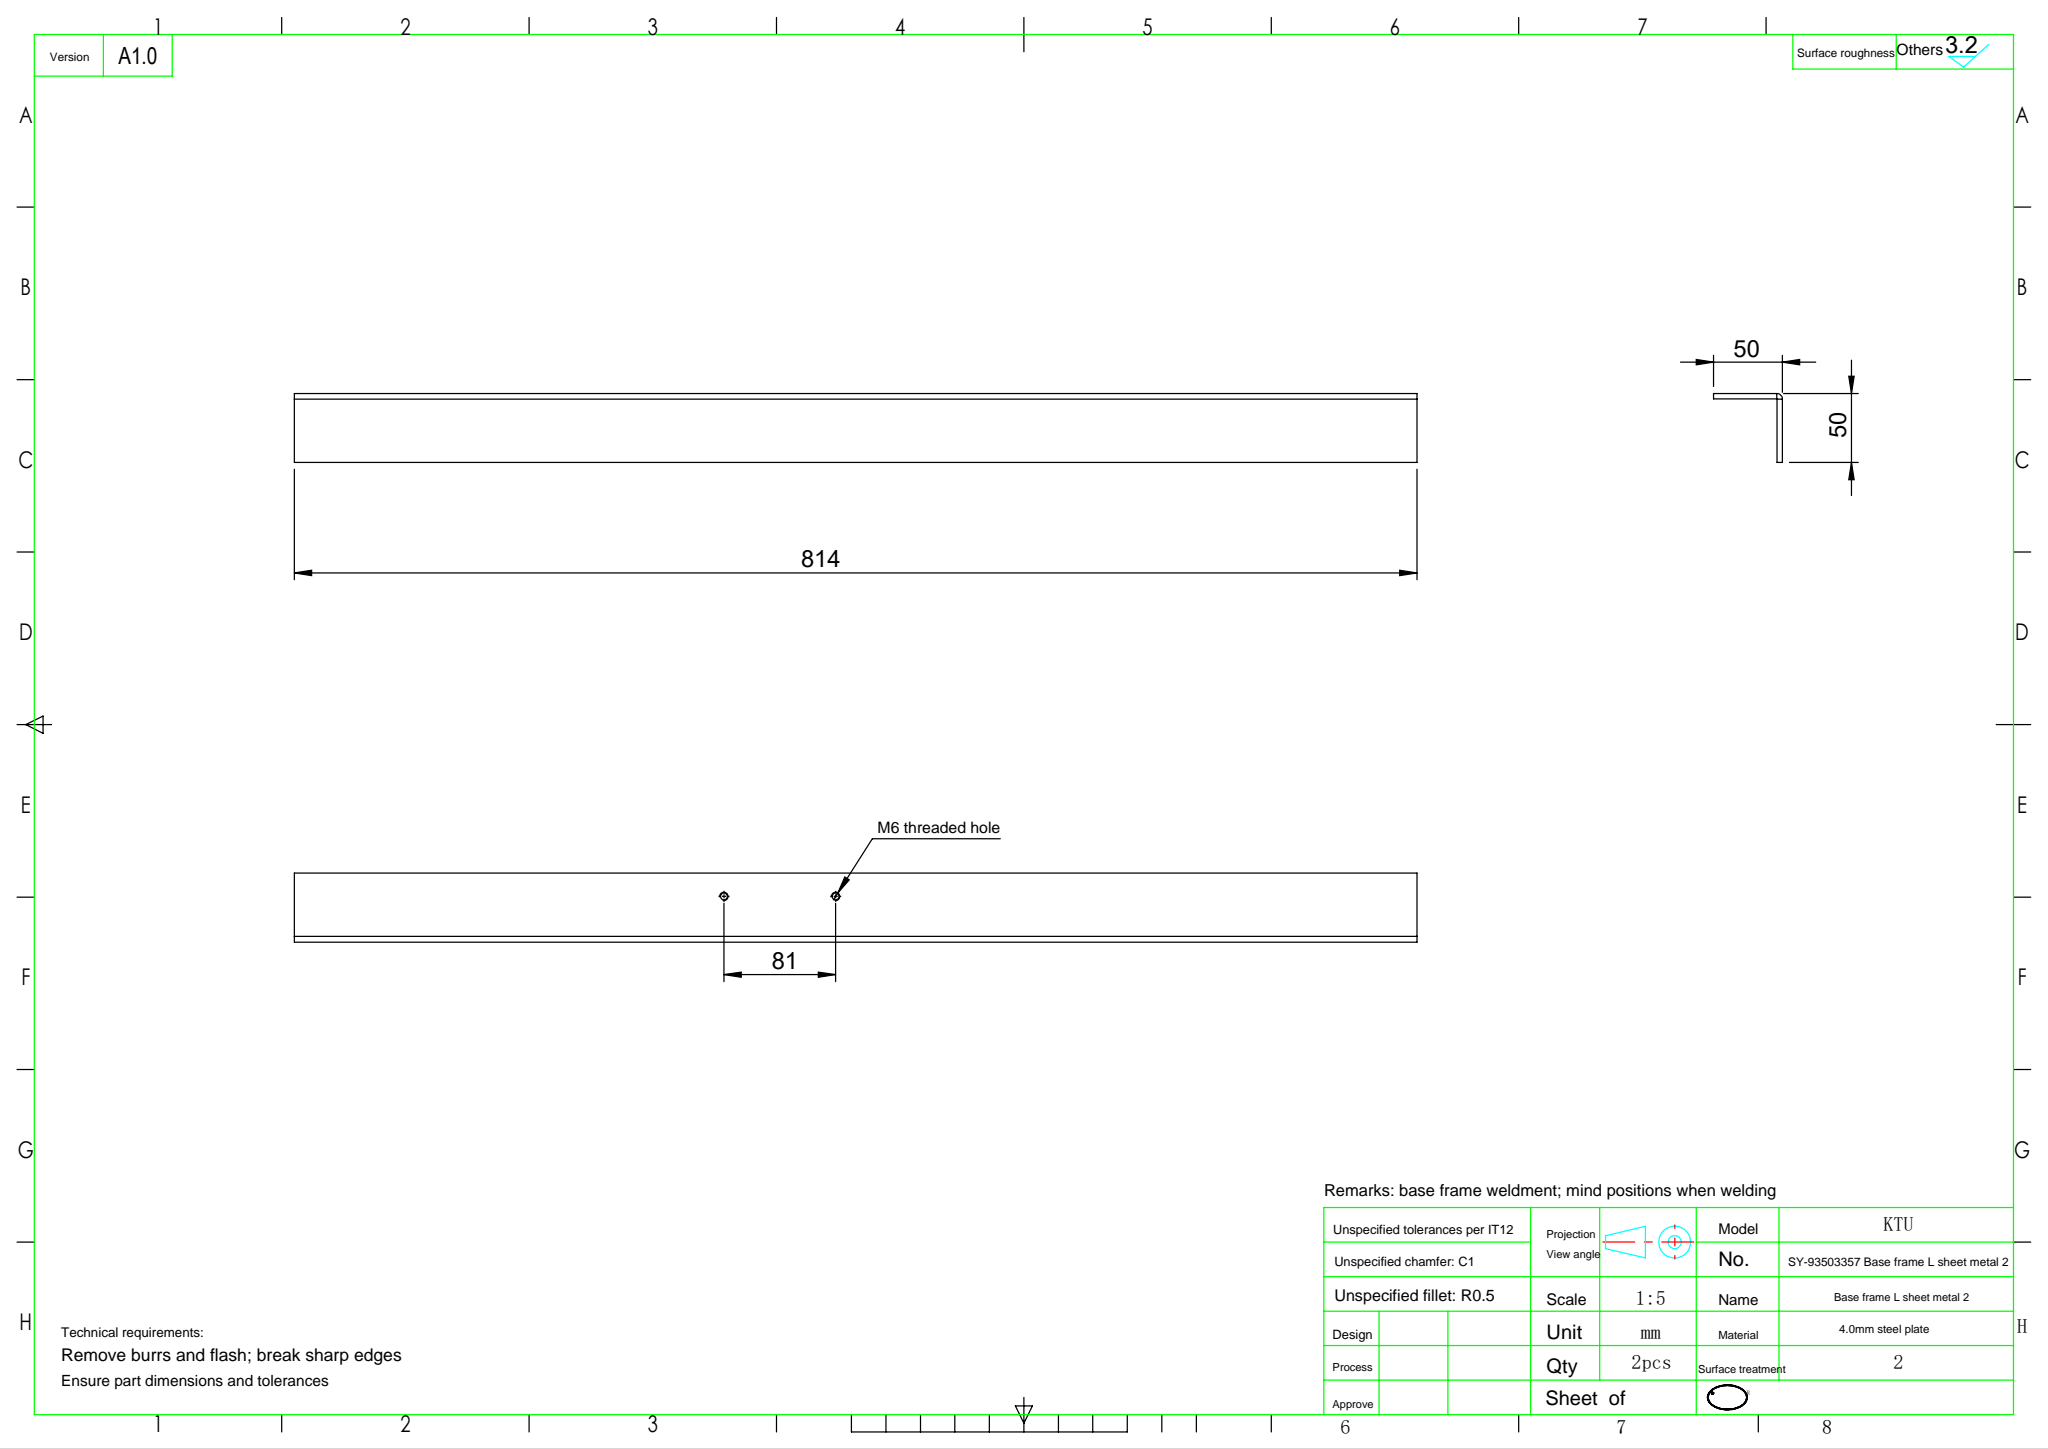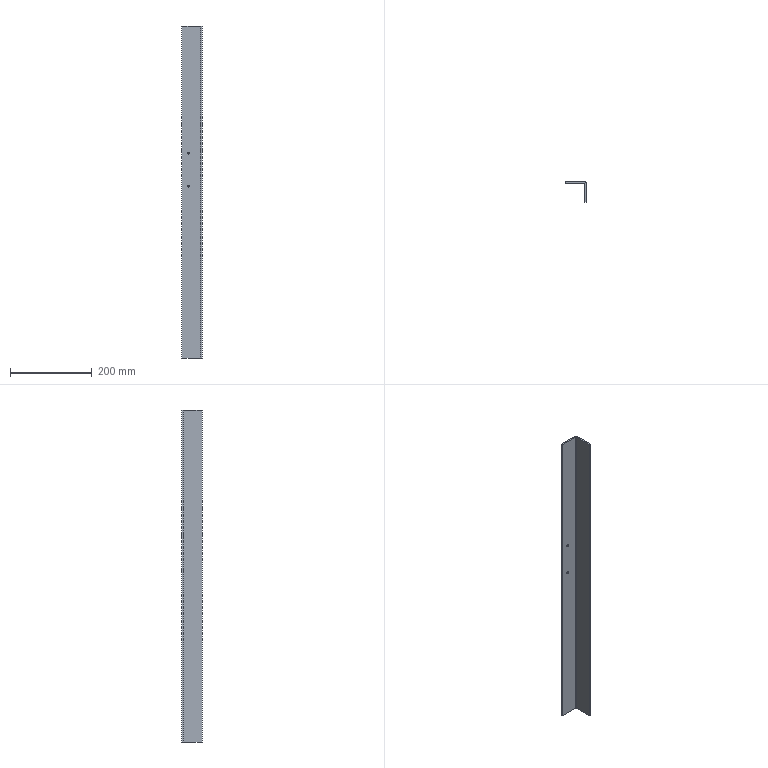Part | SolidWorks | features FlatPattern 1, HoleWzd 1, SMBaseFlange 1, SheetMetal 1 | 1 solid | 18 faces | box 50 x 50 x 814 mm | volume 309344 mm3 | plane 12 | cylinder 6 | commonest cylinder face diameters 5 x4 0.4 x1 8.4 x1
STEP:
#1=CARTESIAN_POINT('',(-33.15,-4.,-309.));
#2=VERTEX_POINT('',#1);
#3=CARTESIAN_POINT('',(-33.15,-4.,-314.));
#4=VERTEX_POINT('',#3);
#5=CARTESIAN_POINT('',(-33.15,-4.,-311.5));
#6=DIRECTION('',(0.,-1.,0.));
#7=DIRECTION('',(0.,0.,-1.));
#8=AXIS2_PLACEMENT_3D('',#5,#6,#7);
#9=CIRCLE('',#8,2.5);
#10=EDGE_CURVE('',#2,#4,#9,.T.);
#11=ORIENTED_EDGE('',*,*,#10,.T.);
#12=CARTESIAN_POINT('',(-33.15,0.,-314.));
#13=VERTEX_POINT('',#12);
#14=CARTESIAN_POINT('',(-33.15,0.,-314.));
#15=DIRECTION('',(0.,1.,0.));
#16=VECTOR('',#15,1000.);
#17=LINE('',#14,#16);
#18=EDGE_CURVE('',#4,#13,#17,.T.);
#19=ORIENTED_EDGE('',*,*,#18,.T.);
#20=CARTESIAN_POINT('',(-33.15,0.,-309.));
#21=VERTEX_POINT('',#20);
#22=CARTESIAN_POINT('',(-33.15,0.,-311.5));
#23=DIRECTION('',(0.,1.,0.));
#24=DIRECTION('',(0.,0.,1.));
#25=AXIS2_PLACEMENT_3D('',#22,#23,#24);
#26=CIRCLE('',#25,2.5);
#27=EDGE_CURVE('',#13,#21,#26,.T.);
#28=ORIENTED_EDGE('',*,*,#27,.T.);
#29=CARTESIAN_POINT('',(-33.15,0.,-309.));
#30=DIRECTION('',(0.,1.,0.));
#31=VECTOR('',#30,1000.);
#32=LINE('',#29,#31);
#33=EDGE_CURVE('',#2,#21,#32,.T.);
#34=ORIENTED_EDGE('',*,*,#33,.F.);
#35=EDGE_LOOP('',(#11,#19,#28,#34));
#36=FACE_OUTER_BOUND('',#35,.T.);
#37=CARTESIAN_POINT('',(-33.15,0.,-311.5));
#38=DIRECTION('',(0.,1.,0.));
#39=DIRECTION('',(0.,0.,1.));
#40=AXIS2_PLACEMENT_3D('',#37,#38,#39);
#41=CYLINDRICAL_SURFACE('',#40,2.5);
#42=ADVANCED_FACE('',(#36),#41,.F.);
#43=CARTESIAN_POINT('',(-33.15,-4.,-390.));
#44=VERTEX_POINT('',#43);
#45=CARTESIAN_POINT('',(-33.15,-4.,-395.));
#46=VERTEX_POINT('',#45);
#47=CARTESIAN_POINT('',(-33.15,-4.,-392.5));
#48=DIRECTION('',(0.,-1.,0.));
#49=DIRECTION('',(0.,0.,-1.));
#50=AXIS2_PLACEMENT_3D('',#47,#48,#49);
#51=CIRCLE('',#50,2.5);
#52=EDGE_CURVE('',#44,#46,#51,.T.);
#53=ORIENTED_EDGE('',*,*,#52,.T.);
#54=CARTESIAN_POINT('',(-33.15,0.,-395.));
#55=VERTEX_POINT('',#54);
#56=CARTESIAN_POINT('',(-33.15,0.,-395.));
#57=DIRECTION('',(0.,1.,0.));
#58=VECTOR('',#57,1000.);
#59=LINE('',#56,#58);
#60=EDGE_CURVE('',#46,#55,#59,.T.);
#61=ORIENTED_EDGE('',*,*,#60,.T.);
#62=CARTESIAN_POINT('',(-33.15,0.,-390.));
#63=VERTEX_POINT('',#62);
#64=CARTESIAN_POINT('',(-33.15,0.,-392.5));
#65=DIRECTION('',(0.,1.,0.));
#66=DIRECTION('',(0.,0.,1.));
#67=AXIS2_PLACEMENT_3D('',#64,#65,#66);
#68=CIRCLE('',#67,2.5);
#69=EDGE_CURVE('',#55,#63,#68,.T.);
#70=ORIENTED_EDGE('',*,*,#69,.T.);
#71=CARTESIAN_POINT('',(-33.15,0.,-390.));
#72=DIRECTION('',(0.,1.,0.));
#73=VECTOR('',#72,1000.);
#74=LINE('',#71,#73);
#75=EDGE_CURVE('',#44,#63,#74,.T.);
#76=ORIENTED_EDGE('',*,*,#75,.F.);
#77=EDGE_LOOP('',(#53,#61,#70,#76));
#78=FACE_OUTER_BOUND('',#77,.T.);
#79=CARTESIAN_POINT('',(-33.15,0.,-392.5));
#80=DIRECTION('',(0.,1.,0.));
#81=DIRECTION('',(0.,0.,1.));
#82=AXIS2_PLACEMENT_3D('',#79,#80,#81);
#83=CYLINDRICAL_SURFACE('',#82,2.5);
#84=ADVANCED_FACE('',(#78),#83,.F.);
#85=CARTESIAN_POINT('',(-4.2,0.,-814.));
#86=VERTEX_POINT('',#85);
#87=CARTESIAN_POINT('',(-4.2,-4.,-814.));
#88=VERTEX_POINT('',#87);
#89=CARTESIAN_POINT('',(-4.2,0.,-814.));
#90=DIRECTION('',(0.,-1.,0.));
#91=VECTOR('',#90,1000.);
#92=LINE('',#89,#91);
#93=EDGE_CURVE('',#86,#88,#92,.T.);
#94=ORIENTED_EDGE('',*,*,#93,.F.);
#95=CARTESIAN_POINT('',(0.,-4.2,-814.));
#96=VERTEX_POINT('',#95);
#97=CARTESIAN_POINT('',(-4.2,-4.2,-814.));
#98=DIRECTION('',(0.,0.,-1.));
#99=DIRECTION('',(1.,0.,0.));
#100=AXIS2_PLACEMENT_3D('',#97,#98,#99);
#101=CIRCLE('',#100,4.2);
#102=EDGE_CURVE('',#86,#96,#101,.T.);
#103=ORIENTED_EDGE('',*,*,#102,.T.);
#104=CARTESIAN_POINT('',(-4.,-4.2,-814.));
#105=VERTEX_POINT('',#104);
#106=CARTESIAN_POINT('',(-4.,-4.2,-814.));
#107=DIRECTION('',(1.,0.,0.));
#108=VECTOR('',#107,1000.);
#109=LINE('',#106,#108);
#110=EDGE_CURVE('',#105,#96,#109,.T.);
#111=ORIENTED_EDGE('',*,*,#110,.F.);
#112=CARTESIAN_POINT('',(-4.2,-4.2,-814.));
#113=DIRECTION('',(0.,0.,-1.));
#114=DIRECTION('',(1.,0.,0.));
#115=AXIS2_PLACEMENT_3D('',#112,#113,#114);
#116=CIRCLE('',#115,0.2);
#117=EDGE_CURVE('',#88,#105,#116,.T.);
#118=ORIENTED_EDGE('',*,*,#117,.F.);
#119=EDGE_LOOP('',(#94,#103,#111,#118));
#120=FACE_OUTER_BOUND('',#119,.T.);
#121=CARTESIAN_POINT('',(-4.2,0.,-814.));
#122=DIRECTION('',(0.,0.,-1.));
#123=DIRECTION('',(-1.,0.,0.));
#124=AXIS2_PLACEMENT_3D('',#121,#122,#123);
#125=PLANE('',#124);
#126=ADVANCED_FACE('',(#120),#125,.T.);
#127=CARTESIAN_POINT('',(-50.,0.,-814.));
#128=VERTEX_POINT('',#127);
#129=CARTESIAN_POINT('',(-50.,0.,-814.));
#130=DIRECTION('',(1.,0.,0.));
#131=VECTOR('',#130,1000.);
#132=LINE('',#129,#131);
#133=EDGE_CURVE('',#128,#86,#132,.T.);
#134=ORIENTED_EDGE('',*,*,#133,.T.);
#135=ORIENTED_EDGE('',*,*,#93,.T.);
#136=CARTESIAN_POINT('',(-50.,-4.,-814.));
#137=VERTEX_POINT('',#136);
#138=CARTESIAN_POINT('',(-50.,-4.,-814.));
#139=DIRECTION('',(1.,0.,0.));
#140=VECTOR('',#139,1000.);
#141=LINE('',#138,#140);
#142=EDGE_CURVE('',#137,#88,#141,.T.);
#143=ORIENTED_EDGE('',*,*,#142,.F.);
#144=CARTESIAN_POINT('',(-50.,-4.,-814.));
#145=DIRECTION('',(0.,1.,0.));
#146=VECTOR('',#145,1000.);
#147=LINE('',#144,#146);
#148=EDGE_CURVE('',#137,#128,#147,.T.);
#149=ORIENTED_EDGE('',*,*,#148,.T.);
#150=EDGE_LOOP('',(#134,#135,#143,#149));
#151=FACE_OUTER_BOUND('',#150,.T.);
#152=CARTESIAN_POINT('',(-4.,-4.2,-814.));
#153=DIRECTION('',(0.,0.,-1.));
#154=DIRECTION('',(-1.,0.,0.));
#155=AXIS2_PLACEMENT_3D('',#152,#153,#154);
#156=PLANE('',#155);
#157=ADVANCED_FACE('',(#151),#156,.T.);
#158=CARTESIAN_POINT('',(0.,-4.2,0.));
#159=VERTEX_POINT('',#158);
#160=CARTESIAN_POINT('',(-4.,-4.2,0.));
#161=VERTEX_POINT('',#160);
#162=CARTESIAN_POINT('',(0.,-4.2,0.));
#163=DIRECTION('',(-1.,0.,0.));
#164=VECTOR('',#163,1000.);
#165=LINE('',#162,#164);
#166=EDGE_CURVE('',#159,#161,#165,.T.);
#167=ORIENTED_EDGE('',*,*,#166,.F.);
#168=CARTESIAN_POINT('',(-4.2,0.,0.));
#169=VERTEX_POINT('',#168);
#170=CARTESIAN_POINT('',(-4.2,-4.2,0.));
#171=DIRECTION('',(0.,0.,-1.));
#172=DIRECTION('',(1.,0.,0.));
#173=AXIS2_PLACEMENT_3D('',#170,#171,#172);
#174=CIRCLE('',#173,4.2);
#175=EDGE_CURVE('',#169,#159,#174,.T.);
#176=ORIENTED_EDGE('',*,*,#175,.F.);
#177=CARTESIAN_POINT('',(-4.2,-4.,0.));
#178=VERTEX_POINT('',#177);
#179=CARTESIAN_POINT('',(-4.2,-4.,0.));
#180=DIRECTION('',(0.,1.,0.));
#181=VECTOR('',#180,1000.);
#182=LINE('',#179,#181);
#183=EDGE_CURVE('',#178,#169,#182,.T.);
#184=ORIENTED_EDGE('',*,*,#183,.F.);
#185=CARTESIAN_POINT('',(-4.2,-4.2,0.));
#186=DIRECTION('',(0.,0.,-1.));
#187=DIRECTION('',(1.,0.,0.));
#188=AXIS2_PLACEMENT_3D('',#185,#186,#187);
#189=CIRCLE('',#188,0.2);
#190=EDGE_CURVE('',#178,#161,#189,.T.);
#191=ORIENTED_EDGE('',*,*,#190,.T.);
#192=EDGE_LOOP('',(#167,#176,#184,#191));
#193=FACE_OUTER_BOUND('',#192,.T.);
#194=CARTESIAN_POINT('',(0.,-4.2,0.));
#195=DIRECTION('',(0.,0.,1.));
#196=DIRECTION('',(1.,0.,0.));
#197=AXIS2_PLACEMENT_3D('',#194,#195,#196);
#198=PLANE('',#197);
#199=ADVANCED_FACE('',(#193),#198,.T.);
#200=CARTESIAN_POINT('',(0.,-50.,0.));
#201=VERTEX_POINT('',#200);
#202=CARTESIAN_POINT('',(0.,0.,0.));
#203=DIRECTION('',(0.,-1.,0.));
#204=VECTOR('',#203,1000.);
#205=LINE('',#202,#204);
#206=EDGE_CURVE('',#159,#201,#205,.T.);
#207=ORIENTED_EDGE('',*,*,#206,.F.);
#208=ORIENTED_EDGE('',*,*,#166,.T.);
#209=CARTESIAN_POINT('',(-4.,-50.,0.));
#210=VERTEX_POINT('',#209);
#211=CARTESIAN_POINT('',(-4.,0.,0.));
#212=DIRECTION('',(0.,-1.,0.));
#213=VECTOR('',#212,1000.);
#214=LINE('',#211,#213);
#215=EDGE_CURVE('',#161,#210,#214,.T.);
#216=ORIENTED_EDGE('',*,*,#215,.T.);
#217=CARTESIAN_POINT('',(0.,-50.,0.));
#218=DIRECTION('',(-1.,0.,0.));
#219=VECTOR('',#218,1000.);
#220=LINE('',#217,#219);
#221=EDGE_CURVE('',#201,#210,#220,.T.);
#222=ORIENTED_EDGE('',*,*,#221,.F.);
#223=EDGE_LOOP('',(#207,#208,#216,#222));
#224=FACE_OUTER_BOUND('',#223,.T.);
#225=CARTESIAN_POINT('',(-4.2,-4.,0.));
#226=DIRECTION('',(0.,0.,1.));
#227=DIRECTION('',(1.,0.,0.));
#228=AXIS2_PLACEMENT_3D('',#225,#226,#227);
#229=PLANE('',#228);
#230=ADVANCED_FACE('',(#224),#229,.T.);
#231=ORIENTED_EDGE('',*,*,#215,.F.);
#232=CARTESIAN_POINT('',(-4.,-4.2,-814.));
#233=DIRECTION('',(0.,0.,1.));
#234=VECTOR('',#233,1000.);
#235=LINE('',#232,#234);
#236=EDGE_CURVE('',#105,#161,#235,.T.);
#237=ORIENTED_EDGE('',*,*,#236,.F.);
#238=CARTESIAN_POINT('',(-4.,-50.,-814.));
#239=VERTEX_POINT('',#238);
#240=CARTESIAN_POINT('',(-4.,0.,-814.));
#241=DIRECTION('',(0.,-1.,0.));
#242=VECTOR('',#241,1000.);
#243=LINE('',#240,#242);
#244=EDGE_CURVE('',#105,#239,#243,.T.);
#245=ORIENTED_EDGE('',*,*,#244,.T.);
#246=CARTESIAN_POINT('',(-4.,-50.,-814.));
#247=DIRECTION('',(0.,0.,1.));
#248=VECTOR('',#247,1000.);
#249=LINE('',#246,#248);
#250=EDGE_CURVE('',#239,#210,#249,.T.);
#251=ORIENTED_EDGE('',*,*,#250,.T.);
#252=EDGE_LOOP('',(#231,#237,#245,#251));
#253=FACE_OUTER_BOUND('',#252,.T.);
#254=CARTESIAN_POINT('',(-4.,0.,-814.));
#255=DIRECTION('',(-1.,0.,0.));
#256=DIRECTION('',(0.,-1.,0.));
#257=AXIS2_PLACEMENT_3D('',#254,#255,#256);
#258=PLANE('',#257);
#259=ADVANCED_FACE('',(#253),#258,.T.);
#260=ORIENTED_EDGE('',*,*,#190,.F.);
#261=CARTESIAN_POINT('',(-4.2,-4.,-814.));
#262=DIRECTION('',(0.,0.,1.));
#263=VECTOR('',#262,1000.);
#264=LINE('',#261,#263);
#265=EDGE_CURVE('',#88,#178,#264,.T.);
#266=ORIENTED_EDGE('',*,*,#265,.F.);
#267=ORIENTED_EDGE('',*,*,#117,.T.);
#268=ORIENTED_EDGE('',*,*,#236,.T.);
#269=EDGE_LOOP('',(#260,#266,#267,#268));
#270=FACE_OUTER_BOUND('',#269,.T.);
#271=CARTESIAN_POINT('',(-4.2,-4.2,-814.));
#272=DIRECTION('',(0.,0.,1.));
#273=DIRECTION('',(1.,0.,0.));
#274=AXIS2_PLACEMENT_3D('',#271,#272,#273);
#275=CYLINDRICAL_SURFACE('',#274,0.2);
#276=ADVANCED_FACE('',(#270),#275,.F.);
#277=ORIENTED_EDGE('',*,*,#10,.F.);
#278=CARTESIAN_POINT('',(-33.15,-4.,-311.5));
#279=DIRECTION('',(0.,-1.,0.));
#280=DIRECTION('',(0.,0.,-1.));
#281=AXIS2_PLACEMENT_3D('',#278,#279,#280);
#282=CIRCLE('',#281,2.5);
#283=EDGE_CURVE('',#4,#2,#282,.T.);
#284=ORIENTED_EDGE('',*,*,#283,.F.);
#285=EDGE_LOOP('',(#277,#284));
#286=FACE_BOUND('',#285,.T.);
#287=ORIENTED_EDGE('',*,*,#52,.F.);
#288=CARTESIAN_POINT('',(-33.15,-4.,-392.5));
#289=DIRECTION('',(0.,-1.,0.));
#290=DIRECTION('',(0.,0.,-1.));
#291=AXIS2_PLACEMENT_3D('',#288,#289,#290);
#292=CIRCLE('',#291,2.5);
#293=EDGE_CURVE('',#46,#44,#292,.T.);
#294=ORIENTED_EDGE('',*,*,#293,.F.);
#295=EDGE_LOOP('',(#287,#294));
#296=FACE_BOUND('',#295,.T.);
#297=CARTESIAN_POINT('',(-50.,-4.,0.));
#298=VERTEX_POINT('',#297);
#299=CARTESIAN_POINT('',(-50.,-4.,0.));
#300=DIRECTION('',(1.,0.,0.));
#301=VECTOR('',#300,1000.);
#302=LINE('',#299,#301);
#303=EDGE_CURVE('',#298,#178,#302,.T.);
#304=ORIENTED_EDGE('',*,*,#303,.F.);
#305=CARTESIAN_POINT('',(-50.,-4.,-814.));
#306=DIRECTION('',(0.,0.,1.));
#307=VECTOR('',#306,1000.);
#308=LINE('',#305,#307);
#309=EDGE_CURVE('',#137,#298,#308,.T.);
#310=ORIENTED_EDGE('',*,*,#309,.F.);
#311=ORIENTED_EDGE('',*,*,#142,.T.);
#312=ORIENTED_EDGE('',*,*,#265,.T.);
#313=EDGE_LOOP('',(#304,#310,#311,#312));
#314=FACE_OUTER_BOUND('',#313,.T.);
#315=CARTESIAN_POINT('',(-50.,-4.,-814.));
#316=DIRECTION('',(0.,-1.,0.));
#317=DIRECTION('',(0.,0.,-1.));
#318=AXIS2_PLACEMENT_3D('',#315,#316,#317);
#319=PLANE('',#318);
#320=ADVANCED_FACE('',(#286,#296,#314),#319,.T.);
#321=CARTESIAN_POINT('',(-50.,0.,0.));
#322=VERTEX_POINT('',#321);
#323=CARTESIAN_POINT('',(-50.,-4.,0.));
#324=DIRECTION('',(0.,1.,0.));
#325=VECTOR('',#324,1000.);
#326=LINE('',#323,#325);
#327=EDGE_CURVE('',#298,#322,#326,.T.);
#328=ORIENTED_EDGE('',*,*,#327,.T.);
#329=CARTESIAN_POINT('',(-50.,0.,-814.));
#330=DIRECTION('',(0.,0.,1.));
#331=VECTOR('',#330,1000.);
#332=LINE('',#329,#331);
#333=EDGE_CURVE('',#128,#322,#332,.T.);
#334=ORIENTED_EDGE('',*,*,#333,.F.);
#335=ORIENTED_EDGE('',*,*,#148,.F.);
#336=ORIENTED_EDGE('',*,*,#309,.T.);
#337=EDGE_LOOP('',(#328,#334,#335,#336));
#338=FACE_OUTER_BOUND('',#337,.T.);
#339=CARTESIAN_POINT('',(-50.,-4.,-814.));
#340=DIRECTION('',(1.,0.,0.));
#341=DIRECTION('',(0.,0.,-1.));
#342=AXIS2_PLACEMENT_3D('',#339,#340,#341);
#343=PLANE('',#342);
#344=ADVANCED_FACE('',(#338),#343,.F.);
#345=CARTESIAN_POINT('',(-33.15,0.,-311.5));
#346=DIRECTION('',(0.,1.,0.));
#347=DIRECTION('',(0.,0.,1.));
#348=AXIS2_PLACEMENT_3D('',#345,#346,#347);
#349=CIRCLE('',#348,2.5);
#350=EDGE_CURVE('',#21,#13,#349,.T.);
#351=ORIENTED_EDGE('',*,*,#350,.F.);
#352=ORIENTED_EDGE('',*,*,#27,.F.);
#353=EDGE_LOOP('',(#351,#352));
#354=FACE_BOUND('',#353,.T.);
#355=CARTESIAN_POINT('',(-33.15,0.,-392.5));
#356=DIRECTION('',(0.,1.,0.));
#357=DIRECTION('',(0.,0.,1.));
#358=AXIS2_PLACEMENT_3D('',#355,#356,#357);
#359=CIRCLE('',#358,2.5);
#360=EDGE_CURVE('',#63,#55,#359,.T.);
#361=ORIENTED_EDGE('',*,*,#360,.F.);
#362=ORIENTED_EDGE('',*,*,#69,.F.);
#363=EDGE_LOOP('',(#361,#362));
#364=FACE_BOUND('',#363,.T.);
#365=CARTESIAN_POINT('',(-50.,0.,0.));
#366=DIRECTION('',(1.,0.,0.));
#367=VECTOR('',#366,1000.);
#368=LINE('',#365,#367);
#369=EDGE_CURVE('',#322,#169,#368,.T.);
#370=ORIENTED_EDGE('',*,*,#369,.T.);
#371=CARTESIAN_POINT('',(-4.2,0.,-814.));
#372=DIRECTION('',(0.,0.,1.));
#373=VECTOR('',#372,1000.);
#374=LINE('',#371,#373);
#375=EDGE_CURVE('',#86,#169,#374,.T.);
#376=ORIENTED_EDGE('',*,*,#375,.F.);
#377=ORIENTED_EDGE('',*,*,#133,.F.);
#378=ORIENTED_EDGE('',*,*,#333,.T.);
#379=EDGE_LOOP('',(#370,#376,#377,#378));
#380=FACE_OUTER_BOUND('',#379,.T.);
#381=CARTESIAN_POINT('',(-50.,0.,-814.));
#382=DIRECTION('',(0.,-1.,0.));
#383=DIRECTION('',(0.,0.,-1.));
#384=AXIS2_PLACEMENT_3D('',#381,#382,#383);
#385=PLANE('',#384);
#386=ADVANCED_FACE('',(#354,#364,#380),#385,.F.);
#387=ORIENTED_EDGE('',*,*,#175,.T.);
#388=CARTESIAN_POINT('',(0.,-4.2,-814.));
#389=DIRECTION('',(0.,0.,1.));
#390=VECTOR('',#389,1000.);
#391=LINE('',#388,#390);
#392=EDGE_CURVE('',#96,#159,#391,.T.);
#393=ORIENTED_EDGE('',*,*,#392,.F.);
#394=ORIENTED_EDGE('',*,*,#102,.F.);
#395=ORIENTED_EDGE('',*,*,#375,.T.);
#396=EDGE_LOOP('',(#387,#393,#394,#395));
#397=FACE_OUTER_BOUND('',#396,.T.);
#398=CARTESIAN_POINT('',(-4.2,-4.2,-814.));
#399=DIRECTION('',(0.,0.,1.));
#400=DIRECTION('',(1.,0.,0.));
#401=AXIS2_PLACEMENT_3D('',#398,#399,#400);
#402=CYLINDRICAL_SURFACE('',#401,4.2);
#403=ADVANCED_FACE('',(#397),#402,.T.);
#404=ORIENTED_EDGE('',*,*,#206,.T.);
#405=CARTESIAN_POINT('',(0.,-50.,-814.));
#406=VERTEX_POINT('',#405);
#407=CARTESIAN_POINT('',(0.,-50.,-814.));
#408=DIRECTION('',(0.,0.,1.));
#409=VECTOR('',#408,1000.);
#410=LINE('',#407,#409);
#411=EDGE_CURVE('',#406,#201,#410,.T.);
#412=ORIENTED_EDGE('',*,*,#411,.F.);
#413=CARTESIAN_POINT('',(0.,0.,-814.));
#414=DIRECTION('',(0.,-1.,0.));
#415=VECTOR('',#414,1000.);
#416=LINE('',#413,#415);
#417=EDGE_CURVE('',#96,#406,#416,.T.);
#418=ORIENTED_EDGE('',*,*,#417,.F.);
#419=ORIENTED_EDGE('',*,*,#392,.T.);
#420=EDGE_LOOP('',(#404,#412,#418,#419));
#421=FACE_OUTER_BOUND('',#420,.T.);
#422=CARTESIAN_POINT('',(0.,0.,-814.));
#423=DIRECTION('',(-1.,0.,0.));
#424=DIRECTION('',(0.,-1.,0.));
#425=AXIS2_PLACEMENT_3D('',#422,#423,#424);
#426=PLANE('',#425);
#427=ADVANCED_FACE('',(#421),#426,.F.);
#428=ORIENTED_EDGE('',*,*,#221,.T.);
#429=ORIENTED_EDGE('',*,*,#250,.F.);
#430=CARTESIAN_POINT('',(0.,-50.,-814.));
#431=DIRECTION('',(-1.,0.,0.));
#432=VECTOR('',#431,1000.);
#433=LINE('',#430,#432);
#434=EDGE_CURVE('',#406,#239,#433,.T.);
#435=ORIENTED_EDGE('',*,*,#434,.F.);
#436=ORIENTED_EDGE('',*,*,#411,.T.);
#437=EDGE_LOOP('',(#428,#429,#435,#436));
#438=FACE_OUTER_BOUND('',#437,.T.);
#439=CARTESIAN_POINT('',(0.,-50.,-814.));
#440=DIRECTION('',(0.,1.,0.));
#441=DIRECTION('',(0.,0.,1.));
#442=AXIS2_PLACEMENT_3D('',#439,#440,#441);
#443=PLANE('',#442);
#444=ADVANCED_FACE('',(#438),#443,.F.);
#445=ORIENTED_EDGE('',*,*,#244,.F.);
#446=ORIENTED_EDGE('',*,*,#110,.T.);
#447=ORIENTED_EDGE('',*,*,#417,.T.);
#448=ORIENTED_EDGE('',*,*,#434,.T.);
#449=EDGE_LOOP('',(#445,#446,#447,#448));
#450=FACE_OUTER_BOUND('',#449,.T.);
#451=CARTESIAN_POINT('',(-4.2,-4.2,-814.));
#452=DIRECTION('',(0.,0.,1.));
#453=DIRECTION('',(1.,0.,0.));
#454=AXIS2_PLACEMENT_3D('',#451,#452,#453);
#455=PLANE('',#454);
#456=ADVANCED_FACE('',(#450),#455,.F.);
#457=ORIENTED_EDGE('',*,*,#303,.T.);
#458=ORIENTED_EDGE('',*,*,#183,.T.);
#459=ORIENTED_EDGE('',*,*,#369,.F.);
#460=ORIENTED_EDGE('',*,*,#327,.F.);
#461=EDGE_LOOP('',(#457,#458,#459,#460));
#462=FACE_OUTER_BOUND('',#461,.T.);
#463=CARTESIAN_POINT('',(-4.2,-4.2,0.));
#464=DIRECTION('',(0.,0.,1.));
#465=DIRECTION('',(1.,0.,0.));
#466=AXIS2_PLACEMENT_3D('',#463,#464,#465);
#467=PLANE('',#466);
#468=ADVANCED_FACE('',(#462),#467,.T.);
#469=ORIENTED_EDGE('',*,*,#60,.F.);
#470=ORIENTED_EDGE('',*,*,#293,.T.);
#471=ORIENTED_EDGE('',*,*,#75,.T.);
#472=ORIENTED_EDGE('',*,*,#360,.T.);
#473=EDGE_LOOP('',(#469,#470,#471,#472));
#474=FACE_OUTER_BOUND('',#473,.T.);
#475=CARTESIAN_POINT('',(-33.15,0.,-392.5));
#476=DIRECTION('',(0.,1.,0.));
#477=DIRECTION('',(0.,0.,1.));
#478=AXIS2_PLACEMENT_3D('',#475,#476,#477);
#479=CYLINDRICAL_SURFACE('',#478,2.5);
#480=ADVANCED_FACE('',(#474),#479,.F.);
#481=ORIENTED_EDGE('',*,*,#18,.F.);
#482=ORIENTED_EDGE('',*,*,#283,.T.);
#483=ORIENTED_EDGE('',*,*,#33,.T.);
#484=ORIENTED_EDGE('',*,*,#350,.T.);
#485=EDGE_LOOP('',(#481,#482,#483,#484));
#486=FACE_OUTER_BOUND('',#485,.T.);
#487=CARTESIAN_POINT('',(-33.15,0.,-311.5));
#488=DIRECTION('',(0.,1.,0.));
#489=DIRECTION('',(0.,0.,1.));
#490=AXIS2_PLACEMENT_3D('',#487,#488,#489);
#491=CYLINDRICAL_SURFACE('',#490,2.5);
#492=ADVANCED_FACE('',(#486),#491,.F.);
#493=CLOSED_SHELL('',(#42,#84,#126,#157,#199,#230,#259,#276,#320,#344,#386,#403,#427,#444,#456,#468,#480,#492));
#494=MANIFOLD_SOLID_BREP('',#493);
#495=CARTESIAN_POINT('',(0.,0.,0.));
#496=DIRECTION('',(0.,0.,1.));
#497=DIRECTION('',(1.,0.,0.));
#498=AXIS2_PLACEMENT_3D('',#495,#496,#497);
#499=(LENGTH_UNIT()NAMED_UNIT(*)SI_UNIT(.MILLI.,.METRE.));
#500=UNCERTAINTY_MEASURE_WITH_UNIT(LENGTH_MEASURE(0.00001),#499,'','');
#501=(NAMED_UNIT(*)PLANE_ANGLE_UNIT()SI_UNIT($,.RADIAN.));
#502=(NAMED_UNIT(*)SI_UNIT($,.STERADIAN.)SOLID_ANGLE_UNIT());
#503=(GEOMETRIC_REPRESENTATION_CONTEXT(3)GLOBAL_UNCERTAINTY_ASSIGNED_CONTEXT((#500))GLOBAL_UNIT_ASSIGNED_CONTEXT((#499,#501,#502))REPRESENTATION_CONTEXT('',''));
#504=ADVANCED_BREP_SHAPE_REPRESENTATION('',(#494,#498),#503);